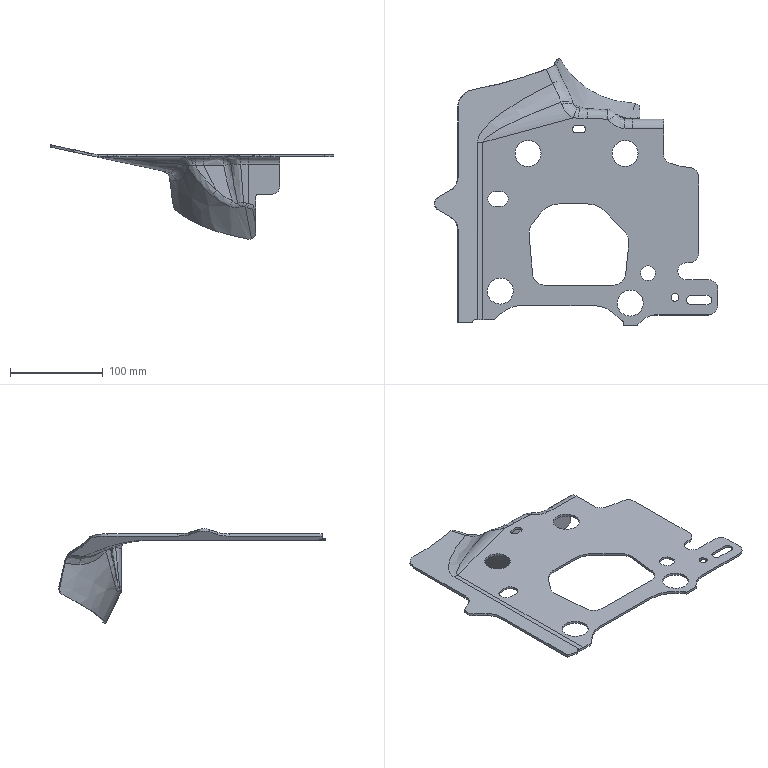Part | STEP file | lll_id178_x_t | 1 solid | 163 faces | box 305 x 286.852 x 101.504 mm | volume 141226 mm3 | spline 100 | plane 44 | cylinder 17 | torus 2 | commonest cylinder face diameters 1 x4 8.05 x2 55 x2 8.55 x1 16 x1 21 x1